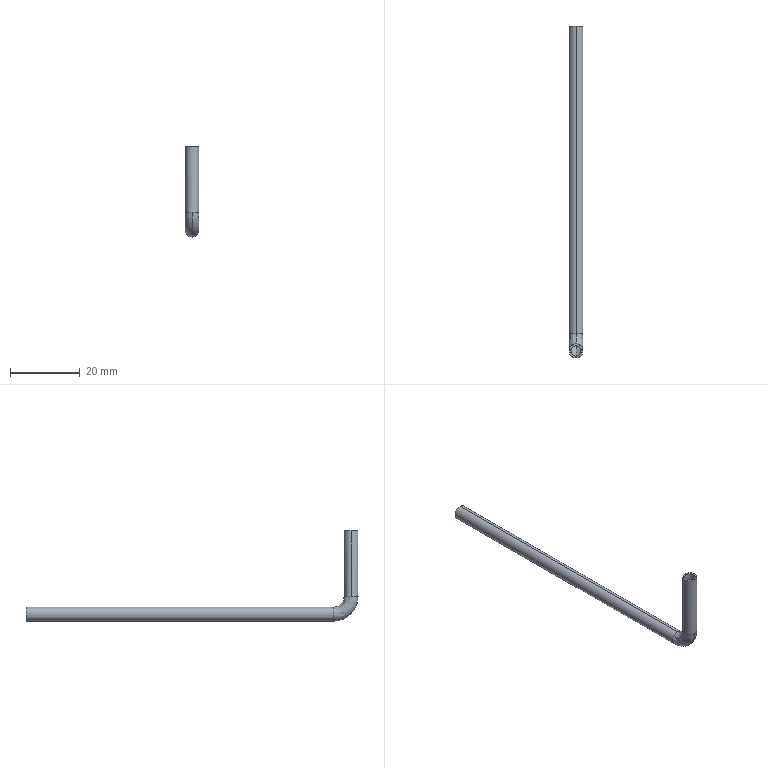Part | SolidWorks | features BaseBody 1 | 1 solid | 14 faces | box 4 x 95.26 x 25.9 mm | volume 632.21 mm3 | cylinder 8 | spline 4 | plane 2 | commonest cylinder face diameters 3 x4 4 x4
STEP:
#1=CARTESIAN_POINT('',(0.,93.26,85.952));
#2=VERTEX_POINT('',#1);
#3=CARTESIAN_POINT('',(0.,93.26,89.952));
#4=VERTEX_POINT('',#3);
#5=CARTESIAN_POINT('',(0.,93.26,87.952));
#6=DIRECTION('',(0.,-1.,0.));
#7=DIRECTION('',(0.,0.,-1.));
#8=AXIS2_PLACEMENT_3D('',#5,#6,#7);
#9=CIRCLE('',#8,2.);
#10=EDGE_CURVE('',#2,#4,#9,.T.);
#11=ORIENTED_EDGE('',*,*,#10,.T.);
#12=CARTESIAN_POINT('',(0.,5.048,89.952));
#13=VERTEX_POINT('',#12);
#14=CARTESIAN_POINT('',(0.,93.26,89.952));
#15=DIRECTION('',(0.,-1.,0.));
#16=VECTOR('',#15,1000.);
#17=LINE('',#14,#16);
#18=EDGE_CURVE('',#4,#13,#17,.T.);
#19=ORIENTED_EDGE('',*,*,#18,.T.);
#20=CARTESIAN_POINT('',(0.,5.048,85.952));
#21=VERTEX_POINT('',#20);
#22=CARTESIAN_POINT('',(0.,5.048,87.952));
#23=DIRECTION('',(0.,1.,0.));
#24=DIRECTION('',(0.,0.,-1.));
#25=AXIS2_PLACEMENT_3D('',#22,#23,#24);
#26=CIRCLE('',#25,2.);
#27=EDGE_CURVE('',#13,#21,#26,.T.);
#28=ORIENTED_EDGE('',*,*,#27,.T.);
#29=CARTESIAN_POINT('',(0.,93.26,85.952));
#30=DIRECTION('',(0.,-1.,0.));
#31=VECTOR('',#30,1000.);
#32=LINE('',#29,#31);
#33=EDGE_CURVE('',#2,#21,#32,.T.);
#34=ORIENTED_EDGE('',*,*,#33,.F.);
#35=EDGE_LOOP('',(#11,#19,#28,#34));
#36=FACE_OUTER_BOUND('',#35,.T.);
#37=CARTESIAN_POINT('',(0.,93.26,87.952));
#38=DIRECTION('',(0.,-1.,0.));
#39=DIRECTION('',(0.,0.,-1.));
#40=AXIS2_PLACEMENT_3D('',#37,#38,#39);
#41=CYLINDRICAL_SURFACE('',#40,2.);
#42=ADVANCED_FACE('',(#36),#41,.T.);
#43=CARTESIAN_POINT('',(-2.,0.,93.));
#44=VERTEX_POINT('',#43);
#45=CARTESIAN_POINT('',(0.,2.,93.));
#46=VERTEX_POINT('',#45);
#47=CARTESIAN_POINT('',(0.,0.,93.));
#48=DIRECTION('',(0.,0.,-1.));
#49=DIRECTION('',(0.,-1.,0.));
#50=AXIS2_PLACEMENT_3D('',#47,#48,#49);
#51=CIRCLE('',#50,2.);
#52=EDGE_CURVE('',#44,#46,#51,.T.);
#53=ORIENTED_EDGE('',*,*,#52,.T.);
#54=CARTESIAN_POINT('',(0.,5.048,93.));
#55=DIRECTION('',(1.,0.,0.));
#56=DIRECTION('',(0.,0.,-1.));
#57=AXIS2_PLACEMENT_3D('',#54,#55,#56);
#58=CIRCLE('',#57,3.048);
#59=EDGE_CURVE('',#46,#13,#58,.T.);
#60=ORIENTED_EDGE('',*,*,#59,.T.);
#61=CARTESIAN_POINT('',(0.,5.048,87.952));
#62=DIRECTION('',(0.,1.,0.));
#63=DIRECTION('',(0.,0.,-1.));
#64=AXIS2_PLACEMENT_3D('',#61,#62,#63);
#65=CIRCLE('',#64,2.);
#66=EDGE_CURVE('',#21,#13,#65,.T.);
#67=ORIENTED_EDGE('',*,*,#66,.F.);
#68=CARTESIAN_POINT('',(0.,-2.,93.));
#69=VERTEX_POINT('',#68);
#70=CARTESIAN_POINT('',(0.,5.048,93.));
#71=DIRECTION('',(1.,0.,0.));
#72=DIRECTION('',(0.,0.,-1.));
#73=AXIS2_PLACEMENT_3D('',#70,#71,#72);
#74=CIRCLE('',#73,7.048);
#75=EDGE_CURVE('',#69,#21,#74,.T.);
#76=ORIENTED_EDGE('',*,*,#75,.F.);
#77=CARTESIAN_POINT('',(0.,0.,93.));
#78=DIRECTION('',(0.,0.,-1.));
#79=DIRECTION('',(0.,-1.,0.));
#80=AXIS2_PLACEMENT_3D('',#77,#78,#79);
#81=CIRCLE('',#80,2.);
#82=EDGE_CURVE('',#69,#44,#81,.T.);
#83=ORIENTED_EDGE('',*,*,#82,.T.);
#84=EDGE_LOOP('',(#53,#60,#67,#76,#83));
#85=FACE_OUTER_BOUND('',#84,.T.);
#86=CARTESIAN_POINT('',(0.,-2.,93.));
#87=CARTESIAN_POINT('',(0.,-2.,88.871));
#88=CARTESIAN_POINT('',(0.,0.9194,85.952));
#89=CARTESIAN_POINT('',(0.,5.048,85.952));
#90=CARTESIAN_POINT('',(-4.,-2.,93.));
#91=CARTESIAN_POINT('',(-4.,-2.,88.871));
#92=CARTESIAN_POINT('',(-4.,0.9194,85.952));
#93=CARTESIAN_POINT('',(-4.,5.048,85.952));
#94=CARTESIAN_POINT('',(-4.,2.,93.));
#95=CARTESIAN_POINT('',(-4.,2.,91.215));
#96=CARTESIAN_POINT('',(-4.,3.263,89.952));
#97=CARTESIAN_POINT('',(-4.,5.048,89.952));
#98=CARTESIAN_POINT('',(0.,2.,93.));
#99=CARTESIAN_POINT('',(0.,2.,91.215));
#100=CARTESIAN_POINT('',(0.,3.263,89.952));
#101=CARTESIAN_POINT('',(0.,5.048,89.952));
#102=(BOUNDED_SURFACE()B_SPLINE_SURFACE(3,3,((#86,#87,#88,#89),(#90,#91,#92,#93),(#94,#95,#96,#97),(#98,#99,#100,#101)),.UNSPECIFIED.,.F.,.F.,.F.)B_SPLINE_SURFACE_WITH_KNOTS((4,4),(4,4),(0.,1.),(0.,1.),.UNSPECIFIED.)GEOMETRIC_REPRESENTATION_ITEM()RATIONAL_B_SPLINE_SURFACE(((1.,0.8047,0.8047,1.),(0.3333,0.2682,0.2682,0.3333),(0.3333,0.2682,0.2682,0.3333),(1.,0.8047,0.8047,1.)))REPRESENTATION_ITEM('')SURFACE());
#103=ADVANCED_FACE('',(#85),#102,.T.);
#104=ORIENTED_EDGE('',*,*,#52,.F.);
#105=CARTESIAN_POINT('',(-2.,0.,111.852));
#106=VERTEX_POINT('',#105);
#107=CARTESIAN_POINT('',(-2.,0.,0.));
#108=DIRECTION('',(0.,0.,1.));
#109=VECTOR('',#108,1000.);
#110=LINE('',#107,#109);
#111=EDGE_CURVE('',#44,#106,#110,.T.);
#112=ORIENTED_EDGE('',*,*,#111,.T.);
#113=CARTESIAN_POINT('',(2.,0.,111.852));
#114=VERTEX_POINT('',#113);
#115=CARTESIAN_POINT('',(0.,0.,111.852));
#116=DIRECTION('',(0.,0.,-1.));
#117=DIRECTION('',(1.,0.,0.));
#118=AXIS2_PLACEMENT_3D('',#115,#116,#117);
#119=CIRCLE('',#118,2.);
#120=EDGE_CURVE('',#106,#114,#119,.T.);
#121=ORIENTED_EDGE('',*,*,#120,.T.);
#122=CARTESIAN_POINT('',(2.,0.,93.));
#123=VERTEX_POINT('',#122);
#124=CARTESIAN_POINT('',(2.,0.,0.));
#125=DIRECTION('',(0.,0.,1.));
#126=VECTOR('',#125,1000.);
#127=LINE('',#124,#126);
#128=EDGE_CURVE('',#123,#114,#127,.T.);
#129=ORIENTED_EDGE('',*,*,#128,.F.);
#130=CARTESIAN_POINT('',(0.,0.,93.));
#131=DIRECTION('',(0.,0.,-1.));
#132=DIRECTION('',(0.,-1.,0.));
#133=AXIS2_PLACEMENT_3D('',#130,#131,#132);
#134=CIRCLE('',#133,2.);
#135=EDGE_CURVE('',#46,#123,#134,.T.);
#136=ORIENTED_EDGE('',*,*,#135,.F.);
#137=EDGE_LOOP('',(#104,#112,#121,#129,#136));
#138=FACE_OUTER_BOUND('',#137,.T.);
#139=CARTESIAN_POINT('',(0.,0.,0.));
#140=DIRECTION('',(0.,0.,1.));
#141=DIRECTION('',(1.,0.,0.));
#142=AXIS2_PLACEMENT_3D('',#139,#140,#141);
#143=CYLINDRICAL_SURFACE('',#142,2.);
#144=ADVANCED_FACE('',(#138),#143,.T.);
#145=CARTESIAN_POINT('',(0.,93.26,89.452));
#146=VERTEX_POINT('',#145);
#147=CARTESIAN_POINT('',(0.,93.26,86.452));
#148=VERTEX_POINT('',#147);
#149=CARTESIAN_POINT('',(0.,93.26,87.952));
#150=DIRECTION('',(0.,-1.,0.));
#151=DIRECTION('',(0.,0.,-1.));
#152=AXIS2_PLACEMENT_3D('',#149,#150,#151);
#153=CIRCLE('',#152,1.5);
#154=EDGE_CURVE('',#146,#148,#153,.T.);
#155=ORIENTED_EDGE('',*,*,#154,.F.);
#156=CARTESIAN_POINT('',(0.,5.048,89.452));
#157=VERTEX_POINT('',#156);
#158=CARTESIAN_POINT('',(0.,93.403,89.452));
#159=DIRECTION('',(0.,-1.,0.));
#160=VECTOR('',#159,1000.);
#161=LINE('',#158,#160);
#162=EDGE_CURVE('',#146,#157,#161,.T.);
#163=ORIENTED_EDGE('',*,*,#162,.T.);
#164=CARTESIAN_POINT('',(0.,5.048,86.452));
#165=VERTEX_POINT('',#164);
#166=CARTESIAN_POINT('',(0.,5.048,87.952));
#167=DIRECTION('',(0.,1.,0.));
#168=DIRECTION('',(0.,0.,-1.));
#169=AXIS2_PLACEMENT_3D('',#166,#167,#168);
#170=CIRCLE('',#169,1.5);
#171=EDGE_CURVE('',#165,#157,#170,.T.);
#172=ORIENTED_EDGE('',*,*,#171,.F.);
#173=CARTESIAN_POINT('',(0.,93.403,86.452));
#174=DIRECTION('',(0.,-1.,0.));
#175=VECTOR('',#174,1000.);
#176=LINE('',#173,#175);
#177=EDGE_CURVE('',#148,#165,#176,.T.);
#178=ORIENTED_EDGE('',*,*,#177,.F.);
#179=EDGE_LOOP('',(#155,#163,#172,#178));
#180=FACE_OUTER_BOUND('',#179,.T.);
#181=CARTESIAN_POINT('',(0.,93.403,87.952));
#182=DIRECTION('',(0.,-1.,0.));
#183=DIRECTION('',(0.,0.,-1.));
#184=AXIS2_PLACEMENT_3D('',#181,#182,#183);
#185=CYLINDRICAL_SURFACE('',#184,1.5);
#186=ADVANCED_FACE('',(#180),#185,.F.);
#187=CARTESIAN_POINT('',(0.,1.5,93.));
#188=VERTEX_POINT('',#187);
#189=CARTESIAN_POINT('',(1.5,0.,93.));
#190=VERTEX_POINT('',#189);
#191=CARTESIAN_POINT('',(0.,0.,93.));
#192=DIRECTION('',(0.,0.,-1.));
#193=DIRECTION('',(0.,-1.,0.));
#194=AXIS2_PLACEMENT_3D('',#191,#192,#193);
#195=CIRCLE('',#194,1.5);
#196=EDGE_CURVE('',#188,#190,#195,.T.);
#197=ORIENTED_EDGE('',*,*,#196,.F.);
#198=CARTESIAN_POINT('',(0.,5.048,93.));
#199=DIRECTION('',(1.,0.,0.));
#200=DIRECTION('',(0.,0.,-1.));
#201=AXIS2_PLACEMENT_3D('',#198,#199,#200);
#202=CIRCLE('',#201,3.548);
#203=EDGE_CURVE('',#188,#157,#202,.T.);
#204=ORIENTED_EDGE('',*,*,#203,.T.);
#205=CARTESIAN_POINT('',(0.,5.048,87.952));
#206=DIRECTION('',(0.,1.,0.));
#207=DIRECTION('',(0.,0.,-1.));
#208=AXIS2_PLACEMENT_3D('',#205,#206,#207);
#209=CIRCLE('',#208,1.5);
#210=EDGE_CURVE('',#157,#165,#209,.T.);
#211=ORIENTED_EDGE('',*,*,#210,.T.);
#212=CARTESIAN_POINT('',(0.,-1.5,93.));
#213=VERTEX_POINT('',#212);
#214=CARTESIAN_POINT('',(0.,5.048,93.));
#215=DIRECTION('',(1.,0.,0.));
#216=DIRECTION('',(0.,0.,-1.));
#217=AXIS2_PLACEMENT_3D('',#214,#215,#216);
#218=CIRCLE('',#217,6.548);
#219=EDGE_CURVE('',#213,#165,#218,.T.);
#220=ORIENTED_EDGE('',*,*,#219,.F.);
#221=CARTESIAN_POINT('',(0.,0.,93.));
#222=DIRECTION('',(0.,0.,-1.));
#223=DIRECTION('',(0.,-1.,0.));
#224=AXIS2_PLACEMENT_3D('',#221,#222,#223);
#225=CIRCLE('',#224,1.5);
#226=EDGE_CURVE('',#190,#213,#225,.T.);
#227=ORIENTED_EDGE('',*,*,#226,.F.);
#228=EDGE_LOOP('',(#197,#204,#211,#220,#227));
#229=FACE_OUTER_BOUND('',#228,.T.);
#230=CARTESIAN_POINT('',(0.,1.5,93.));
#231=CARTESIAN_POINT('',(0.,1.5,90.922));
#232=CARTESIAN_POINT('',(0.,2.97,89.452));
#233=CARTESIAN_POINT('',(0.,5.048,89.452));
#234=CARTESIAN_POINT('',(3.,1.5,93.));
#235=CARTESIAN_POINT('',(3.,1.5,90.922));
#236=CARTESIAN_POINT('',(3.,2.97,89.452));
#237=CARTESIAN_POINT('',(3.,5.048,89.452));
#238=CARTESIAN_POINT('',(3.,-1.5,93.));
#239=CARTESIAN_POINT('',(3.,-1.5,89.164));
#240=CARTESIAN_POINT('',(3.,1.212,86.452));
#241=CARTESIAN_POINT('',(3.,5.048,86.452));
#242=CARTESIAN_POINT('',(0.,-1.5,93.));
#243=CARTESIAN_POINT('',(0.,-1.5,89.164));
#244=CARTESIAN_POINT('',(0.,1.212,86.452));
#245=CARTESIAN_POINT('',(0.,5.048,86.452));
#246=(BOUNDED_SURFACE()B_SPLINE_SURFACE(3,3,((#230,#231,#232,#233),(#234,#235,#236,#237),(#238,#239,#240,#241),(#242,#243,#244,#245)),.UNSPECIFIED.,.F.,.F.,.F.)B_SPLINE_SURFACE_WITH_KNOTS((4,4),(4,4),(0.,1.),(0.,1.),.UNSPECIFIED.)GEOMETRIC_REPRESENTATION_ITEM()RATIONAL_B_SPLINE_SURFACE(((1.,0.8047,0.8047,1.),(0.3333,0.2682,0.2682,0.3333),(0.3333,0.2682,0.2682,0.3333),(1.,0.8047,0.8047,1.)))REPRESENTATION_ITEM('')SURFACE());
#247=ADVANCED_FACE('',(#229),#246,.F.);
#248=ORIENTED_EDGE('',*,*,#226,.T.);
#249=CARTESIAN_POINT('',(-1.5,0.,93.));
#250=VERTEX_POINT('',#249);
#251=CARTESIAN_POINT('',(0.,0.,93.));
#252=DIRECTION('',(0.,0.,-1.));
#253=DIRECTION('',(0.,-1.,0.));
#254=AXIS2_PLACEMENT_3D('',#251,#252,#253);
#255=CIRCLE('',#254,1.5);
#256=EDGE_CURVE('',#213,#250,#255,.T.);
#257=ORIENTED_EDGE('',*,*,#256,.T.);
#258=CARTESIAN_POINT('',(-1.5,0.,111.852));
#259=VERTEX_POINT('',#258);
#260=CARTESIAN_POINT('',(-1.5,0.,-0.143));
#261=DIRECTION('',(0.,0.,1.));
#262=VECTOR('',#261,1000.);
#263=LINE('',#260,#262);
#264=EDGE_CURVE('',#250,#259,#263,.T.);
#265=ORIENTED_EDGE('',*,*,#264,.T.);
#266=CARTESIAN_POINT('',(1.5,0.,111.852));
#267=VERTEX_POINT('',#266);
#268=CARTESIAN_POINT('',(0.,0.,111.852));
#269=DIRECTION('',(0.,0.,1.));
#270=DIRECTION('',(1.,0.,0.));
#271=AXIS2_PLACEMENT_3D('',#268,#269,#270);
#272=CIRCLE('',#271,1.5);
#273=EDGE_CURVE('',#259,#267,#272,.T.);
#274=ORIENTED_EDGE('',*,*,#273,.T.);
#275=CARTESIAN_POINT('',(1.5,0.,-0.143));
#276=DIRECTION('',(0.,0.,1.));
#277=VECTOR('',#276,1000.);
#278=LINE('',#275,#277);
#279=EDGE_CURVE('',#190,#267,#278,.T.);
#280=ORIENTED_EDGE('',*,*,#279,.F.);
#281=EDGE_LOOP('',(#248,#257,#265,#274,#280));
#282=FACE_OUTER_BOUND('',#281,.T.);
#283=CARTESIAN_POINT('',(0.,0.,-0.143));
#284=DIRECTION('',(0.,0.,1.));
#285=DIRECTION('',(1.,0.,0.));
#286=AXIS2_PLACEMENT_3D('',#283,#284,#285);
#287=CYLINDRICAL_SURFACE('',#286,1.5);
#288=ADVANCED_FACE('',(#282),#287,.F.);
#289=ORIENTED_EDGE('',*,*,#18,.F.);
#290=CARTESIAN_POINT('',(0.,93.26,87.952));
#291=DIRECTION('',(0.,-1.,0.));
#292=DIRECTION('',(0.,0.,-1.));
#293=AXIS2_PLACEMENT_3D('',#290,#291,#292);
#294=CIRCLE('',#293,2.);
#295=EDGE_CURVE('',#4,#2,#294,.T.);
#296=ORIENTED_EDGE('',*,*,#295,.T.);
#297=ORIENTED_EDGE('',*,*,#33,.T.);
#298=ORIENTED_EDGE('',*,*,#66,.T.);
#299=EDGE_LOOP('',(#289,#296,#297,#298));
#300=FACE_OUTER_BOUND('',#299,.T.);
#301=CARTESIAN_POINT('',(0.,93.26,87.952));
#302=DIRECTION('',(0.,-1.,0.));
#303=DIRECTION('',(0.,0.,-1.));
#304=AXIS2_PLACEMENT_3D('',#301,#302,#303);
#305=CYLINDRICAL_SURFACE('',#304,2.);
#306=ADVANCED_FACE('',(#300),#305,.T.);
#307=ORIENTED_EDGE('',*,*,#59,.F.);
#308=ORIENTED_EDGE('',*,*,#135,.T.);
#309=CARTESIAN_POINT('',(0.,0.,93.));
#310=DIRECTION('',(0.,0.,-1.));
#311=DIRECTION('',(0.,-1.,0.));
#312=AXIS2_PLACEMENT_3D('',#309,#310,#311);
#313=CIRCLE('',#312,2.);
#314=EDGE_CURVE('',#123,#69,#313,.T.);
#315=ORIENTED_EDGE('',*,*,#314,.T.);
#316=ORIENTED_EDGE('',*,*,#75,.T.);
#317=ORIENTED_EDGE('',*,*,#27,.F.);
#318=EDGE_LOOP('',(#307,#308,#315,#316,#317));
#319=FACE_OUTER_BOUND('',#318,.T.);
#320=CARTESIAN_POINT('',(0.,2.,93.));
#321=CARTESIAN_POINT('',(0.,2.,91.215));
#322=CARTESIAN_POINT('',(0.,3.263,89.952));
#323=CARTESIAN_POINT('',(0.,5.048,89.952));
#324=CARTESIAN_POINT('',(4.,2.,93.));
#325=CARTESIAN_POINT('',(4.,2.,91.215));
#326=CARTESIAN_POINT('',(4.,3.263,89.952));
#327=CARTESIAN_POINT('',(4.,5.048,89.952));
#328=CARTESIAN_POINT('',(4.,-2.,93.));
#329=CARTESIAN_POINT('',(4.,-2.,88.871));
#330=CARTESIAN_POINT('',(4.,0.9194,85.952));
#331=CARTESIAN_POINT('',(4.,5.048,85.952));
#332=CARTESIAN_POINT('',(0.,-2.,93.));
#333=CARTESIAN_POINT('',(0.,-2.,88.871));
#334=CARTESIAN_POINT('',(0.,0.9194,85.952));
#335=CARTESIAN_POINT('',(0.,5.048,85.952));
#336=(BOUNDED_SURFACE()B_SPLINE_SURFACE(3,3,((#320,#321,#322,#323),(#324,#325,#326,#327),(#328,#329,#330,#331),(#332,#333,#334,#335)),.UNSPECIFIED.,.F.,.F.,.F.)B_SPLINE_SURFACE_WITH_KNOTS((4,4),(4,4),(0.,1.),(0.,1.),.UNSPECIFIED.)GEOMETRIC_REPRESENTATION_ITEM()RATIONAL_B_SPLINE_SURFACE(((1.,0.8047,0.8047,1.),(0.3333,0.2682,0.2682,0.3333),(0.3333,0.2682,0.2682,0.3333),(1.,0.8047,0.8047,1.)))REPRESENTATION_ITEM('')SURFACE());
#337=ADVANCED_FACE('',(#319),#336,.T.);
#338=CARTESIAN_POINT('',(0.,93.26,87.952));
#339=DIRECTION('',(0.,-1.,0.));
#340=DIRECTION('',(0.,0.,-1.));
#341=AXIS2_PLACEMENT_3D('',#338,#339,#340);
#342=CIRCLE('',#341,1.5);
#343=EDGE_CURVE('',#148,#146,#342,.T.);
#344=ORIENTED_EDGE('',*,*,#343,.T.);
#345=ORIENTED_EDGE('',*,*,#154,.T.);
#346=EDGE_LOOP('',(#344,#345));
#347=FACE_BOUND('',#346,.T.);
#348=ORIENTED_EDGE('',*,*,#10,.F.);
#349=ORIENTED_EDGE('',*,*,#295,.F.);
#350=EDGE_LOOP('',(#348,#349));
#351=FACE_OUTER_BOUND('',#350,.T.);
#352=CARTESIAN_POINT('',(0.,93.26,87.952));
#353=DIRECTION('',(0.,1.,0.));
#354=DIRECTION('',(0.,0.,1.));
#355=AXIS2_PLACEMENT_3D('',#352,#353,#354);
#356=PLANE('',#355);
#357=ADVANCED_FACE('',(#347,#351),#356,.T.);
#358=ORIENTED_EDGE('',*,*,#111,.F.);
#359=ORIENTED_EDGE('',*,*,#82,.F.);
#360=ORIENTED_EDGE('',*,*,#314,.F.);
#361=ORIENTED_EDGE('',*,*,#128,.T.);
#362=CARTESIAN_POINT('',(0.,0.,111.852));
#363=DIRECTION('',(0.,0.,-1.));
#364=DIRECTION('',(1.,0.,0.));
#365=AXIS2_PLACEMENT_3D('',#362,#363,#364);
#366=CIRCLE('',#365,2.);
#367=EDGE_CURVE('',#114,#106,#366,.T.);
#368=ORIENTED_EDGE('',*,*,#367,.T.);
#369=EDGE_LOOP('',(#358,#359,#360,#361,#368));
#370=FACE_OUTER_BOUND('',#369,.T.);
#371=CARTESIAN_POINT('',(0.,0.,0.));
#372=DIRECTION('',(0.,0.,1.));
#373=DIRECTION('',(1.,0.,0.));
#374=AXIS2_PLACEMENT_3D('',#371,#372,#373);
#375=CYLINDRICAL_SURFACE('',#374,2.);
#376=ADVANCED_FACE('',(#370),#375,.T.);
#377=ORIENTED_EDGE('',*,*,#162,.F.);
#378=ORIENTED_EDGE('',*,*,#343,.F.);
#379=ORIENTED_EDGE('',*,*,#177,.T.);
#380=ORIENTED_EDGE('',*,*,#210,.F.);
#381=EDGE_LOOP('',(#377,#378,#379,#380));
#382=FACE_OUTER_BOUND('',#381,.T.);
#383=CARTESIAN_POINT('',(0.,93.403,87.952));
#384=DIRECTION('',(0.,-1.,0.));
#385=DIRECTION('',(0.,0.,-1.));
#386=AXIS2_PLACEMENT_3D('',#383,#384,#385);
#387=CYLINDRICAL_SURFACE('',#386,1.5);
#388=ADVANCED_FACE('',(#382),#387,.F.);
#389=CARTESIAN_POINT('',(0.,0.,111.852));
#390=DIRECTION('',(0.,0.,1.));
#391=DIRECTION('',(1.,0.,0.));
#392=AXIS2_PLACEMENT_3D('',#389,#390,#391);
#393=CIRCLE('',#392,1.5);
#394=EDGE_CURVE('',#267,#259,#393,.T.);
#395=ORIENTED_EDGE('',*,*,#394,.F.);
#396=ORIENTED_EDGE('',*,*,#273,.F.);
#397=EDGE_LOOP('',(#395,#396));
#398=FACE_BOUND('',#397,.T.);
#399=ORIENTED_EDGE('',*,*,#367,.F.);
#400=ORIENTED_EDGE('',*,*,#120,.F.);
#401=EDGE_LOOP('',(#399,#400));
#402=FACE_OUTER_BOUND('',#401,.T.);
#403=CARTESIAN_POINT('',(0.,0.,111.852));
#404=DIRECTION('',(0.,0.,-1.));
#405=DIRECTION('',(-1.,0.,0.));
#406=AXIS2_PLACEMENT_3D('',#403,#404,#405);
#407=PLANE('',#406);
#408=ADVANCED_FACE('',(#398,#402),#407,.F.);
#409=ORIENTED_EDGE('',*,*,#203,.F.);
#410=CARTESIAN_POINT('',(0.,0.,93.));
#411=DIRECTION('',(0.,0.,-1.));
#412=DIRECTION('',(0.,-1.,0.));
#413=AXIS2_PLACEMENT_3D('',#410,#411,#412);
#414=CIRCLE('',#413,1.5);
#415=EDGE_CURVE('',#250,#188,#414,.T.);
#416=ORIENTED_EDGE('',*,*,#415,.F.);
#417=ORIENTED_EDGE('',*,*,#256,.F.);
#418=ORIENTED_EDGE('',*,*,#219,.T.);
#419=ORIENTED_EDGE('',*,*,#171,.T.);
#420=EDGE_LOOP('',(#409,#416,#417,#418,#419));
#421=FACE_OUTER_BOUND('',#420,.T.);
#422=CARTESIAN_POINT('',(0.,-1.5,93.));
#423=CARTESIAN_POINT('',(0.,-1.5,89.164));
#424=CARTESIAN_POINT('',(0.,1.212,86.452));
#425=CARTESIAN_POINT('',(0.,5.048,86.452));
#426=CARTESIAN_POINT('',(-3.,-1.5,93.));
#427=CARTESIAN_POINT('',(-3.,-1.5,89.164));
#428=CARTESIAN_POINT('',(-3.,1.212,86.452));
#429=CARTESIAN_POINT('',(-3.,5.048,86.452));
#430=CARTESIAN_POINT('',(-3.,1.5,93.));
#431=CARTESIAN_POINT('',(-3.,1.5,90.922));
#432=CARTESIAN_POINT('',(-3.,2.97,89.452));
#433=CARTESIAN_POINT('',(-3.,5.048,89.452));
#434=CARTESIAN_POINT('',(0.,1.5,93.));
#435=CARTESIAN_POINT('',(0.,1.5,90.922));
#436=CARTESIAN_POINT('',(0.,2.97,89.452));
#437=CARTESIAN_POINT('',(0.,5.048,89.452));
#438=(BOUNDED_SURFACE()B_SPLINE_SURFACE(3,3,((#422,#423,#424,#425),(#426,#427,#428,#429),(#430,#431,#432,#433),(#434,#435,#436,#437)),.UNSPECIFIED.,.F.,.F.,.T.)B_SPLINE_SURFACE_WITH_KNOTS((4,4),(4,4),(0.,1.),(0.,1.),.UNSPECIFIED.)GEOMETRIC_REPRESENTATION_ITEM()RATIONAL_B_SPLINE_SURFACE(((1.,0.8047,0.8047,1.),(0.3333,0.2682,0.2682,0.3333),(0.3333,0.2682,0.2682,0.3333),(1.,0.8047,0.8047,1.)))REPRESENTATION_ITEM('')SURFACE());
#439=ADVANCED_FACE('',(#421),#438,.F.);
#440=ORIENTED_EDGE('',*,*,#264,.F.);
#441=ORIENTED_EDGE('',*,*,#415,.T.);
#442=ORIENTED_EDGE('',*,*,#196,.T.);
#443=ORIENTED_EDGE('',*,*,#279,.T.);
#444=ORIENTED_EDGE('',*,*,#394,.T.);
#445=EDGE_LOOP('',(#440,#441,#442,#443,#444));
#446=FACE_OUTER_BOUND('',#445,.T.);
#447=CARTESIAN_POINT('',(0.,0.,-0.143));
#448=DIRECTION('',(0.,0.,1.));
#449=DIRECTION('',(1.,0.,0.));
#450=AXIS2_PLACEMENT_3D('',#447,#448,#449);
#451=CYLINDRICAL_SURFACE('',#450,1.5);
#452=ADVANCED_FACE('',(#446),#451,.F.);
#453=CLOSED_SHELL('',(#42,#103,#144,#186,#247,#288,#306,#337,#357,#376,#388,#408,#439,#452));
#454=MANIFOLD_SOLID_BREP('',#453);
#455=CARTESIAN_POINT('',(0.,0.,0.));
#456=DIRECTION('',(0.,0.,1.));
#457=DIRECTION('',(1.,0.,0.));
#458=AXIS2_PLACEMENT_3D('',#455,#456,#457);
#459=(LENGTH_UNIT()NAMED_UNIT(*)SI_UNIT(.MILLI.,.METRE.));
#460=UNCERTAINTY_MEASURE_WITH_UNIT(LENGTH_MEASURE(0.00001),#459,'','');
#461=(NAMED_UNIT(*)PLANE_ANGLE_UNIT()SI_UNIT($,.RADIAN.));
#462=(NAMED_UNIT(*)SI_UNIT($,.STERADIAN.)SOLID_ANGLE_UNIT());
#463=(GEOMETRIC_REPRESENTATION_CONTEXT(3)GLOBAL_UNCERTAINTY_ASSIGNED_CONTEXT((#460))GLOBAL_UNIT_ASSIGNED_CONTEXT((#459,#461,#462))REPRESENTATION_CONTEXT('',''));
#464=ADVANCED_BREP_SHAPE_REPRESENTATION('',(#454,#458),#463);